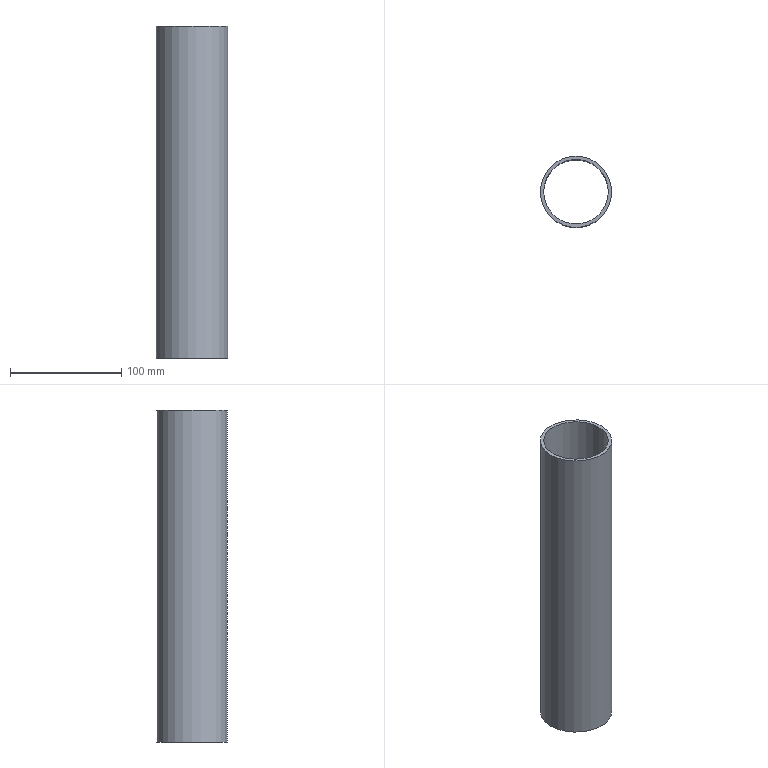Part | STEP file | JBJ-P-1000-08 | 1 solid | 4 faces | box 64 x 64 x 298 mm | volume 171324 mm3 | plane 2 | cylinder 2 | commonest cylinder face diameters 58 x1 64 x1
STEP:
#1=CARTESIAN_POINT('',(32.,0.,298.));
#2=VERTEX_POINT('',#1);
#3=CARTESIAN_POINT('',(0.,0.,298.));
#4=DIRECTION('',(0.,0.,1.));
#5=DIRECTION('',(1.,0.,0.));
#6=AXIS2_PLACEMENT_3D('',#3,#4,#5);
#7=CIRCLE('',#6,32.);
#8=EDGE_CURVE('',#2,#2,#7,.T.);
#9=ORIENTED_EDGE('',*,*,#8,.T.);
#10=EDGE_LOOP('',(#9));
#11=FACE_OUTER_BOUND('',#10,.T.);
#12=CARTESIAN_POINT('',(29.,0.,298.));
#13=VERTEX_POINT('',#12);
#14=CARTESIAN_POINT('',(0.,0.,298.));
#15=DIRECTION('',(0.,0.,1.));
#16=DIRECTION('',(1.,0.,0.));
#17=AXIS2_PLACEMENT_3D('',#14,#15,#16);
#18=CIRCLE('',#17,29.);
#19=EDGE_CURVE('',#13,#13,#18,.T.);
#20=ORIENTED_EDGE('',*,*,#19,.F.);
#21=EDGE_LOOP('',(#20));
#22=FACE_BOUND('',#21,.T.);
#23=CARTESIAN_POINT('',(0.,0.,298.));
#24=DIRECTION('',(0.,0.,1.));
#25=DIRECTION('',(1.,0.,0.));
#26=AXIS2_PLACEMENT_3D('',#23,#24,#25);
#27=PLANE('',#26);
#28=ADVANCED_FACE('',(#11,#22),#27,.T.);
#29=CARTESIAN_POINT('',(32.,0.,0.));
#30=VERTEX_POINT('',#29);
#31=CARTESIAN_POINT('',(0.,0.,0.));
#32=DIRECTION('',(0.,0.,1.));
#33=DIRECTION('',(1.,0.,0.));
#34=AXIS2_PLACEMENT_3D('',#31,#32,#33);
#35=CIRCLE('',#34,32.);
#36=EDGE_CURVE('',#30,#30,#35,.T.);
#37=ORIENTED_EDGE('',*,*,#36,.F.);
#38=EDGE_LOOP('',(#37));
#39=FACE_OUTER_BOUND('',#38,.T.);
#40=CARTESIAN_POINT('',(29.,0.,0.));
#41=VERTEX_POINT('',#40);
#42=CARTESIAN_POINT('',(0.,0.,0.));
#43=DIRECTION('',(0.,0.,1.));
#44=DIRECTION('',(1.,0.,0.));
#45=AXIS2_PLACEMENT_3D('',#42,#43,#44);
#46=CIRCLE('',#45,29.);
#47=EDGE_CURVE('',#41,#41,#46,.T.);
#48=ORIENTED_EDGE('',*,*,#47,.T.);
#49=EDGE_LOOP('',(#48));
#50=FACE_BOUND('',#49,.T.);
#51=CARTESIAN_POINT('',(0.,0.,0.));
#52=DIRECTION('',(0.,0.,1.));
#53=DIRECTION('',(1.,0.,0.));
#54=AXIS2_PLACEMENT_3D('',#51,#52,#53);
#55=PLANE('',#54);
#56=ADVANCED_FACE('',(#39,#50),#55,.F.);
#57=ORIENTED_EDGE('',*,*,#8,.F.);
#58=EDGE_LOOP('',(#57));
#59=FACE_OUTER_BOUND('',#58,.T.);
#60=ORIENTED_EDGE('',*,*,#36,.T.);
#61=EDGE_LOOP('',(#60));
#62=FACE_OUTER_BOUND('',#61,.T.);
#63=CARTESIAN_POINT('',(0.,0.,298.));
#64=DIRECTION('',(0.,0.,-1.));
#65=DIRECTION('',(-1.,0.,0.));
#66=AXIS2_PLACEMENT_3D('',#63,#64,#65);
#67=CYLINDRICAL_SURFACE('',#66,32.);
#68=ADVANCED_FACE('',(#59,#62),#67,.T.);
#69=ORIENTED_EDGE('',*,*,#19,.T.);
#70=EDGE_LOOP('',(#69));
#71=FACE_OUTER_BOUND('',#70,.T.);
#72=ORIENTED_EDGE('',*,*,#47,.F.);
#73=EDGE_LOOP('',(#72));
#74=FACE_OUTER_BOUND('',#73,.T.);
#75=CARTESIAN_POINT('',(0.,0.,298.));
#76=DIRECTION('',(0.,0.,-1.));
#77=DIRECTION('',(-1.,0.,0.));
#78=AXIS2_PLACEMENT_3D('',#75,#76,#77);
#79=CYLINDRICAL_SURFACE('',#78,29.);
#80=ADVANCED_FACE('',(#71,#74),#79,.F.);
#81=CLOSED_SHELL('',(#28,#56,#68,#80));
#82=MANIFOLD_SOLID_BREP('',#81);
#83=CARTESIAN_POINT('',(0.,0.,0.));
#84=DIRECTION('',(0.,0.,1.));
#85=DIRECTION('',(1.,0.,0.));
#86=AXIS2_PLACEMENT_3D('',#83,#84,#85);
#87=(LENGTH_UNIT()NAMED_UNIT(*)SI_UNIT(.MILLI.,.METRE.));
#88=UNCERTAINTY_MEASURE_WITH_UNIT(LENGTH_MEASURE(0.00001),#87,'','');
#89=(NAMED_UNIT(*)PLANE_ANGLE_UNIT()SI_UNIT($,.RADIAN.));
#90=(NAMED_UNIT(*)SI_UNIT($,.STERADIAN.)SOLID_ANGLE_UNIT());
#91=(GEOMETRIC_REPRESENTATION_CONTEXT(3)GLOBAL_UNCERTAINTY_ASSIGNED_CONTEXT((#88))GLOBAL_UNIT_ASSIGNED_CONTEXT((#87,#89,#90))REPRESENTATION_CONTEXT('',''));
#92=ADVANCED_BREP_SHAPE_REPRESENTATION('',(#82,#86),#91);